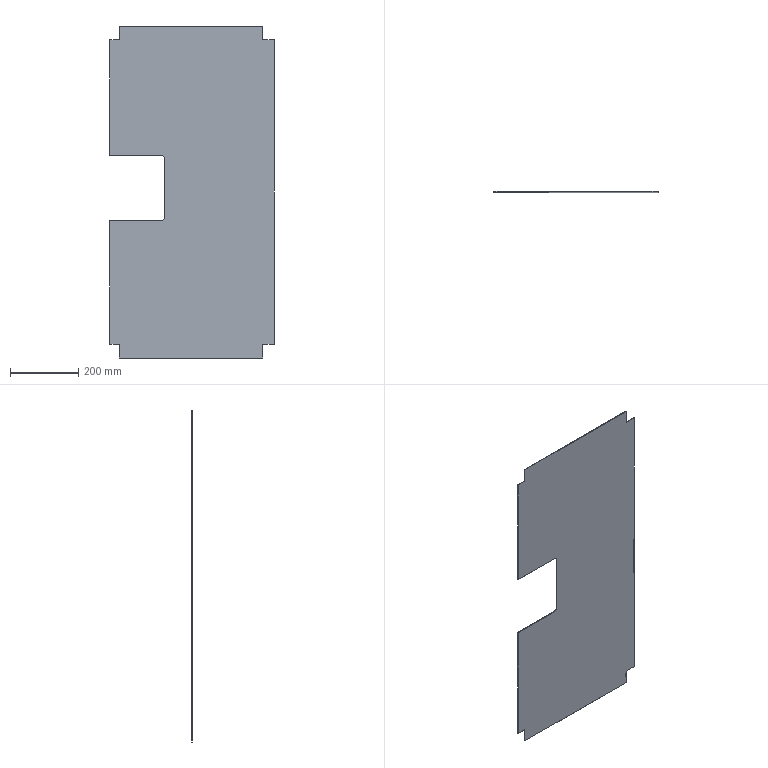Part | SolidWorks | features BaseBody 1 | 1 solid | 20 faces | box 480 x 1.5 x 970 mm | volume 645737 mm3 | plane 18 | cylinder 2 | commonest cylinder face diameters 20 x2
STEP:
#1=CARTESIAN_POINT('',(-254.,-1.5,-83.686));
#2=VERTEX_POINT('',#1);
#3=CARTESIAN_POINT('',(-104.677,-1.5,-83.686));
#4=VERTEX_POINT('',#3);
#5=CARTESIAN_POINT('',(0.,-1.5,-83.686));
#6=DIRECTION('',(1.,0.,0.));
#7=VECTOR('',#6,1000.);
#8=LINE('',#5,#7);
#9=EDGE_CURVE('',#2,#4,#8,.T.);
#10=ORIENTED_EDGE('',*,*,#9,.F.);
#11=CARTESIAN_POINT('',(-254.,-1.5,-445.));
#12=VERTEX_POINT('',#11);
#13=CARTESIAN_POINT('',(-254.,-1.5,0.));
#14=DIRECTION('',(0.,0.,1.));
#15=VECTOR('',#14,1000.);
#16=LINE('',#13,#15);
#17=EDGE_CURVE('',#12,#2,#16,.T.);
#18=ORIENTED_EDGE('',*,*,#17,.F.);
#19=CARTESIAN_POINT('',(-226.,-1.5,-445.));
#20=VERTEX_POINT('',#19);
#21=CARTESIAN_POINT('',(0.,-1.5,-445.));
#22=DIRECTION('',(-1.,0.,0.));
#23=VECTOR('',#22,1000.);
#24=LINE('',#21,#23);
#25=EDGE_CURVE('',#20,#12,#24,.T.);
#26=ORIENTED_EDGE('',*,*,#25,.F.);
#27=CARTESIAN_POINT('',(-226.,-1.5,-485.));
#28=VERTEX_POINT('',#27);
#29=CARTESIAN_POINT('',(-226.,-1.5,0.));
#30=DIRECTION('',(0.,0.,1.));
#31=VECTOR('',#30,1000.);
#32=LINE('',#29,#31);
#33=EDGE_CURVE('',#28,#20,#32,.T.);
#34=ORIENTED_EDGE('',*,*,#33,.F.);
#35=CARTESIAN_POINT('',(193.,-1.5,-485.));
#36=VERTEX_POINT('',#35);
#37=CARTESIAN_POINT('',(0.,-1.5,-485.));
#38=DIRECTION('',(-1.,0.,0.));
#39=VECTOR('',#38,1000.);
#40=LINE('',#37,#39);
#41=EDGE_CURVE('',#36,#28,#40,.T.);
#42=ORIENTED_EDGE('',*,*,#41,.F.);
#43=CARTESIAN_POINT('',(193.,-1.5,-445.));
#44=VERTEX_POINT('',#43);
#45=CARTESIAN_POINT('',(193.,-1.5,0.));
#46=DIRECTION('',(0.,0.,-1.));
#47=VECTOR('',#46,1000.);
#48=LINE('',#45,#47);
#49=EDGE_CURVE('',#44,#36,#48,.T.);
#50=ORIENTED_EDGE('',*,*,#49,.F.);
#51=CARTESIAN_POINT('',(226.,-1.5,-445.));
#52=VERTEX_POINT('',#51);
#53=CARTESIAN_POINT('',(0.,-1.5,-445.));
#54=DIRECTION('',(-1.,0.,0.));
#55=VECTOR('',#54,1000.);
#56=LINE('',#53,#55);
#57=EDGE_CURVE('',#52,#44,#56,.T.);
#58=ORIENTED_EDGE('',*,*,#57,.F.);
#59=CARTESIAN_POINT('',(226.,-1.5,445.));
#60=VERTEX_POINT('',#59);
#61=CARTESIAN_POINT('',(226.,-1.5,0.));
#62=DIRECTION('',(0.,0.,-1.));
#63=VECTOR('',#62,1000.);
#64=LINE('',#61,#63);
#65=EDGE_CURVE('',#60,#52,#64,.T.);
#66=ORIENTED_EDGE('',*,*,#65,.F.);
#67=CARTESIAN_POINT('',(193.,-1.5,445.));
#68=VERTEX_POINT('',#67);
#69=CARTESIAN_POINT('',(0.,-1.5,445.));
#70=DIRECTION('',(1.,0.,0.));
#71=VECTOR('',#70,1000.);
#72=LINE('',#69,#71);
#73=EDGE_CURVE('',#68,#60,#72,.T.);
#74=ORIENTED_EDGE('',*,*,#73,.F.);
#75=CARTESIAN_POINT('',(193.,-1.5,485.));
#76=VERTEX_POINT('',#75);
#77=CARTESIAN_POINT('',(193.,-1.5,0.));
#78=DIRECTION('',(0.,0.,-1.));
#79=VECTOR('',#78,1000.);
#80=LINE('',#77,#79);
#81=EDGE_CURVE('',#76,#68,#80,.T.);
#82=ORIENTED_EDGE('',*,*,#81,.F.);
#83=CARTESIAN_POINT('',(-226.,-1.5,485.));
#84=VERTEX_POINT('',#83);
#85=CARTESIAN_POINT('',(0.,-1.5,485.));
#86=DIRECTION('',(1.,0.,0.));
#87=VECTOR('',#86,1000.);
#88=LINE('',#85,#87);
#89=EDGE_CURVE('',#84,#76,#88,.T.);
#90=ORIENTED_EDGE('',*,*,#89,.F.);
#91=CARTESIAN_POINT('',(-226.,-1.5,445.));
#92=VERTEX_POINT('',#91);
#93=CARTESIAN_POINT('',(-226.,-1.5,0.));
#94=DIRECTION('',(0.,0.,1.));
#95=VECTOR('',#94,1000.);
#96=LINE('',#93,#95);
#97=EDGE_CURVE('',#92,#84,#96,.T.);
#98=ORIENTED_EDGE('',*,*,#97,.F.);
#99=CARTESIAN_POINT('',(-254.,-1.5,445.));
#100=VERTEX_POINT('',#99);
#101=CARTESIAN_POINT('',(0.,-1.5,445.));
#102=DIRECTION('',(1.,0.,0.));
#103=VECTOR('',#102,1000.);
#104=LINE('',#101,#103);
#105=EDGE_CURVE('',#100,#92,#104,.T.);
#106=ORIENTED_EDGE('',*,*,#105,.F.);
#107=CARTESIAN_POINT('',(-254.,-1.5,106.314));
#108=VERTEX_POINT('',#107);
#109=CARTESIAN_POINT('',(-254.,-1.5,0.));
#110=DIRECTION('',(0.,0.,1.));
#111=VECTOR('',#110,1000.);
#112=LINE('',#109,#111);
#113=EDGE_CURVE('',#108,#100,#112,.T.);
#114=ORIENTED_EDGE('',*,*,#113,.F.);
#115=CARTESIAN_POINT('',(-104.677,-1.5,106.314));
#116=VERTEX_POINT('',#115);
#117=CARTESIAN_POINT('',(0.,-1.5,106.314));
#118=DIRECTION('',(-1.,0.,0.));
#119=VECTOR('',#118,1000.);
#120=LINE('',#117,#119);
#121=EDGE_CURVE('',#116,#108,#120,.T.);
#122=ORIENTED_EDGE('',*,*,#121,.F.);
#123=CARTESIAN_POINT('',(-94.677,-1.5,96.314));
#124=VERTEX_POINT('',#123);
#125=CARTESIAN_POINT('',(-104.677,-1.5,96.314));
#126=DIRECTION('',(0.,-1.,0.));
#127=DIRECTION('',(0.,0.,1.));
#128=AXIS2_PLACEMENT_3D('',#125,#126,#127);
#129=CIRCLE('',#128,10.);
#130=EDGE_CURVE('',#124,#116,#129,.T.);
#131=ORIENTED_EDGE('',*,*,#130,.F.);
#132=CARTESIAN_POINT('',(-94.677,-1.5,-73.686));
#133=VERTEX_POINT('',#132);
#134=CARTESIAN_POINT('',(-94.677,-1.5,0.));
#135=DIRECTION('',(0.,0.,1.));
#136=VECTOR('',#135,1000.);
#137=LINE('',#134,#136);
#138=EDGE_CURVE('',#133,#124,#137,.T.);
#139=ORIENTED_EDGE('',*,*,#138,.F.);
#140=CARTESIAN_POINT('',(-104.677,-1.5,-73.686));
#141=DIRECTION('',(0.,-1.,0.));
#142=DIRECTION('',(0.,0.,1.));
#143=AXIS2_PLACEMENT_3D('',#140,#141,#142);
#144=CIRCLE('',#143,10.);
#145=EDGE_CURVE('',#4,#133,#144,.T.);
#146=ORIENTED_EDGE('',*,*,#145,.F.);
#147=EDGE_LOOP('',(#10,#18,#26,#34,#42,#50,#58,#66,#74,#82,#90,#98,#106,#114,#122,#131,#139,#146));
#148=FACE_OUTER_BOUND('',#147,.T.);
#149=CARTESIAN_POINT('',(0.,-1.5,0.));
#150=DIRECTION('',(0.,1.,0.));
#151=DIRECTION('',(0.,0.,1.));
#152=AXIS2_PLACEMENT_3D('',#149,#150,#151);
#153=PLANE('',#152);
#154=ADVANCED_FACE('',(#148),#153,.F.);
#155=CARTESIAN_POINT('',(-104.677,0.,-83.686));
#156=VERTEX_POINT('',#155);
#157=CARTESIAN_POINT('',(-94.677,0.,-73.686));
#158=VERTEX_POINT('',#157);
#159=CARTESIAN_POINT('',(-104.677,0.,-73.686));
#160=DIRECTION('',(0.,-1.,0.));
#161=DIRECTION('',(0.,0.,1.));
#162=AXIS2_PLACEMENT_3D('',#159,#160,#161);
#163=CIRCLE('',#162,10.);
#164=EDGE_CURVE('',#156,#158,#163,.T.);
#165=ORIENTED_EDGE('',*,*,#164,.F.);
#166=CARTESIAN_POINT('',(-104.677,-10.,-83.686));
#167=DIRECTION('',(0.,1.,0.));
#168=VECTOR('',#167,1000.);
#169=LINE('',#166,#168);
#170=EDGE_CURVE('',#4,#156,#169,.T.);
#171=ORIENTED_EDGE('',*,*,#170,.F.);
#172=ORIENTED_EDGE('',*,*,#145,.T.);
#173=CARTESIAN_POINT('',(-94.677,-10.,-73.686));
#174=DIRECTION('',(0.,-1.,0.));
#175=VECTOR('',#174,1000.);
#176=LINE('',#173,#175);
#177=EDGE_CURVE('',#158,#133,#176,.T.);
#178=ORIENTED_EDGE('',*,*,#177,.F.);
#179=EDGE_LOOP('',(#165,#171,#172,#178));
#180=FACE_OUTER_BOUND('',#179,.T.);
#181=CARTESIAN_POINT('',(-104.677,-10.,-73.686));
#182=DIRECTION('',(0.,1.,0.));
#183=DIRECTION('',(0.,0.,1.));
#184=AXIS2_PLACEMENT_3D('',#181,#182,#183);
#185=CYLINDRICAL_SURFACE('',#184,10.);
#186=ADVANCED_FACE('',(#180),#185,.F.);
#187=ORIENTED_EDGE('',*,*,#9,.T.);
#188=ORIENTED_EDGE('',*,*,#170,.T.);
#189=CARTESIAN_POINT('',(-254.,0.,-83.686));
#190=VERTEX_POINT('',#189);
#191=CARTESIAN_POINT('',(-104.677,0.,-83.686));
#192=DIRECTION('',(1.,0.,0.));
#193=VECTOR('',#192,1000.);
#194=LINE('',#191,#193);
#195=EDGE_CURVE('',#190,#156,#194,.T.);
#196=ORIENTED_EDGE('',*,*,#195,.F.);
#197=CARTESIAN_POINT('',(-254.,-10.,-83.686));
#198=DIRECTION('',(0.,1.,0.));
#199=VECTOR('',#198,1000.);
#200=LINE('',#197,#199);
#201=EDGE_CURVE('',#2,#190,#200,.T.);
#202=ORIENTED_EDGE('',*,*,#201,.F.);
#203=EDGE_LOOP('',(#187,#188,#196,#202));
#204=FACE_OUTER_BOUND('',#203,.T.);
#205=CARTESIAN_POINT('',(-104.677,-10.,-83.686));
#206=DIRECTION('',(0.,0.,-1.));
#207=DIRECTION('',(-1.,0.,0.));
#208=AXIS2_PLACEMENT_3D('',#205,#206,#207);
#209=PLANE('',#208);
#210=ADVANCED_FACE('',(#204),#209,.F.);
#211=CARTESIAN_POINT('',(-254.,0.,-445.));
#212=VERTEX_POINT('',#211);
#213=CARTESIAN_POINT('',(-254.,-1.5,-445.));
#214=DIRECTION('',(0.,-1.,0.));
#215=VECTOR('',#214,1000.);
#216=LINE('',#213,#215);
#217=EDGE_CURVE('',#212,#12,#216,.T.);
#218=ORIENTED_EDGE('',*,*,#217,.T.);
#219=ORIENTED_EDGE('',*,*,#17,.T.);
#220=ORIENTED_EDGE('',*,*,#201,.T.);
#221=CARTESIAN_POINT('',(-254.,0.,445.));
#222=DIRECTION('',(0.,0.,-1.));
#223=VECTOR('',#222,1000.);
#224=LINE('',#221,#223);
#225=EDGE_CURVE('',#190,#212,#224,.T.);
#226=ORIENTED_EDGE('',*,*,#225,.T.);
#227=EDGE_LOOP('',(#218,#219,#220,#226));
#228=FACE_OUTER_BOUND('',#227,.T.);
#229=CARTESIAN_POINT('',(-254.,-1.5,445.));
#230=DIRECTION('',(-1.,0.,0.));
#231=DIRECTION('',(0.,0.,1.));
#232=AXIS2_PLACEMENT_3D('',#229,#230,#231);
#233=PLANE('',#232);
#234=ADVANCED_FACE('',(#228),#233,.T.);
#235=ORIENTED_EDGE('',*,*,#25,.T.);
#236=ORIENTED_EDGE('',*,*,#217,.F.);
#237=CARTESIAN_POINT('',(-226.,0.,-445.));
#238=VERTEX_POINT('',#237);
#239=CARTESIAN_POINT('',(-254.,0.,-445.));
#240=DIRECTION('',(1.,0.,0.));
#241=VECTOR('',#240,1000.);
#242=LINE('',#239,#241);
#243=EDGE_CURVE('',#212,#238,#242,.T.);
#244=ORIENTED_EDGE('',*,*,#243,.T.);
#245=CARTESIAN_POINT('',(-226.,-1.5,-445.));
#246=DIRECTION('',(0.,-1.,0.));
#247=VECTOR('',#246,1000.);
#248=LINE('',#245,#247);
#249=EDGE_CURVE('',#238,#20,#248,.T.);
#250=ORIENTED_EDGE('',*,*,#249,.T.);
#251=EDGE_LOOP('',(#235,#236,#244,#250));
#252=FACE_OUTER_BOUND('',#251,.T.);
#253=CARTESIAN_POINT('',(-254.,-1.5,-445.));
#254=DIRECTION('',(0.,0.,-1.));
#255=DIRECTION('',(-1.,0.,0.));
#256=AXIS2_PLACEMENT_3D('',#253,#254,#255);
#257=PLANE('',#256);
#258=ADVANCED_FACE('',(#252),#257,.T.);
#259=ORIENTED_EDGE('',*,*,#33,.T.);
#260=ORIENTED_EDGE('',*,*,#249,.F.);
#261=CARTESIAN_POINT('',(-226.,0.,-485.));
#262=VERTEX_POINT('',#261);
#263=CARTESIAN_POINT('',(-226.,0.,-445.));
#264=DIRECTION('',(0.,0.,-1.));
#265=VECTOR('',#264,1000.);
#266=LINE('',#263,#265);
#267=EDGE_CURVE('',#238,#262,#266,.T.);
#268=ORIENTED_EDGE('',*,*,#267,.T.);
#269=CARTESIAN_POINT('',(-226.,-1.5,-485.));
#270=DIRECTION('',(0.,-1.,0.));
#271=VECTOR('',#270,1000.);
#272=LINE('',#269,#271);
#273=EDGE_CURVE('',#262,#28,#272,.T.);
#274=ORIENTED_EDGE('',*,*,#273,.T.);
#275=EDGE_LOOP('',(#259,#260,#268,#274));
#276=FACE_OUTER_BOUND('',#275,.T.);
#277=CARTESIAN_POINT('',(-226.,-1.5,-445.));
#278=DIRECTION('',(-1.,0.,0.));
#279=DIRECTION('',(0.,0.,1.));
#280=AXIS2_PLACEMENT_3D('',#277,#278,#279);
#281=PLANE('',#280);
#282=ADVANCED_FACE('',(#276),#281,.T.);
#283=ORIENTED_EDGE('',*,*,#41,.T.);
#284=ORIENTED_EDGE('',*,*,#273,.F.);
#285=CARTESIAN_POINT('',(193.,0.,-485.));
#286=VERTEX_POINT('',#285);
#287=CARTESIAN_POINT('',(-226.,0.,-485.));
#288=DIRECTION('',(1.,0.,0.));
#289=VECTOR('',#288,1000.);
#290=LINE('',#287,#289);
#291=EDGE_CURVE('',#262,#286,#290,.T.);
#292=ORIENTED_EDGE('',*,*,#291,.T.);
#293=CARTESIAN_POINT('',(193.,-1.5,-485.));
#294=DIRECTION('',(0.,-1.,0.));
#295=VECTOR('',#294,1000.);
#296=LINE('',#293,#295);
#297=EDGE_CURVE('',#286,#36,#296,.T.);
#298=ORIENTED_EDGE('',*,*,#297,.T.);
#299=EDGE_LOOP('',(#283,#284,#292,#298));
#300=FACE_OUTER_BOUND('',#299,.T.);
#301=CARTESIAN_POINT('',(-226.,-1.5,-485.));
#302=DIRECTION('',(0.,0.,-1.));
#303=DIRECTION('',(-1.,0.,0.));
#304=AXIS2_PLACEMENT_3D('',#301,#302,#303);
#305=PLANE('',#304);
#306=ADVANCED_FACE('',(#300),#305,.T.);
#307=ORIENTED_EDGE('',*,*,#49,.T.);
#308=ORIENTED_EDGE('',*,*,#297,.F.);
#309=CARTESIAN_POINT('',(193.,0.,-445.));
#310=VERTEX_POINT('',#309);
#311=CARTESIAN_POINT('',(193.,0.,-485.));
#312=DIRECTION('',(0.,0.,1.));
#313=VECTOR('',#312,1000.);
#314=LINE('',#311,#313);
#315=EDGE_CURVE('',#286,#310,#314,.T.);
#316=ORIENTED_EDGE('',*,*,#315,.T.);
#317=CARTESIAN_POINT('',(193.,-1.5,-445.));
#318=DIRECTION('',(0.,-1.,0.));
#319=VECTOR('',#318,1000.);
#320=LINE('',#317,#319);
#321=EDGE_CURVE('',#310,#44,#320,.T.);
#322=ORIENTED_EDGE('',*,*,#321,.T.);
#323=EDGE_LOOP('',(#307,#308,#316,#322));
#324=FACE_OUTER_BOUND('',#323,.T.);
#325=CARTESIAN_POINT('',(193.,-1.5,-485.));
#326=DIRECTION('',(1.,0.,0.));
#327=DIRECTION('',(0.,0.,-1.));
#328=AXIS2_PLACEMENT_3D('',#325,#326,#327);
#329=PLANE('',#328);
#330=ADVANCED_FACE('',(#324),#329,.T.);
#331=ORIENTED_EDGE('',*,*,#57,.T.);
#332=ORIENTED_EDGE('',*,*,#321,.F.);
#333=CARTESIAN_POINT('',(226.,0.,-445.));
#334=VERTEX_POINT('',#333);
#335=CARTESIAN_POINT('',(226.,0.,-445.));
#336=DIRECTION('',(1.,0.,0.));
#337=VECTOR('',#336,1000.);
#338=LINE('',#335,#337);
#339=EDGE_CURVE('',#310,#334,#338,.T.);
#340=ORIENTED_EDGE('',*,*,#339,.T.);
#341=CARTESIAN_POINT('',(226.,-1.5,-445.));
#342=DIRECTION('',(0.,-1.,0.));
#343=VECTOR('',#342,1000.);
#344=LINE('',#341,#343);
#345=EDGE_CURVE('',#334,#52,#344,.T.);
#346=ORIENTED_EDGE('',*,*,#345,.T.);
#347=EDGE_LOOP('',(#331,#332,#340,#346));
#348=FACE_OUTER_BOUND('',#347,.T.);
#349=CARTESIAN_POINT('',(226.,-1.5,-445.));
#350=DIRECTION('',(0.,0.,-1.));
#351=DIRECTION('',(-1.,0.,0.));
#352=AXIS2_PLACEMENT_3D('',#349,#350,#351);
#353=PLANE('',#352);
#354=ADVANCED_FACE('',(#348),#353,.T.);
#355=ORIENTED_EDGE('',*,*,#65,.T.);
#356=ORIENTED_EDGE('',*,*,#345,.F.);
#357=CARTESIAN_POINT('',(226.,0.,445.));
#358=VERTEX_POINT('',#357);
#359=CARTESIAN_POINT('',(226.,0.,445.));
#360=DIRECTION('',(0.,0.,1.));
#361=VECTOR('',#360,1000.);
#362=LINE('',#359,#361);
#363=EDGE_CURVE('',#334,#358,#362,.T.);
#364=ORIENTED_EDGE('',*,*,#363,.T.);
#365=CARTESIAN_POINT('',(226.,-1.5,445.));
#366=DIRECTION('',(0.,-1.,0.));
#367=VECTOR('',#366,1000.);
#368=LINE('',#365,#367);
#369=EDGE_CURVE('',#358,#60,#368,.T.);
#370=ORIENTED_EDGE('',*,*,#369,.T.);
#371=EDGE_LOOP('',(#355,#356,#364,#370));
#372=FACE_OUTER_BOUND('',#371,.T.);
#373=CARTESIAN_POINT('',(226.,-1.5,445.));
#374=DIRECTION('',(1.,0.,0.));
#375=DIRECTION('',(0.,0.,-1.));
#376=AXIS2_PLACEMENT_3D('',#373,#374,#375);
#377=PLANE('',#376);
#378=ADVANCED_FACE('',(#372),#377,.T.);
#379=ORIENTED_EDGE('',*,*,#73,.T.);
#380=ORIENTED_EDGE('',*,*,#369,.F.);
#381=CARTESIAN_POINT('',(193.,0.,445.));
#382=VERTEX_POINT('',#381);
#383=CARTESIAN_POINT('',(226.,0.,445.));
#384=DIRECTION('',(-1.,0.,0.));
#385=VECTOR('',#384,1000.);
#386=LINE('',#383,#385);
#387=EDGE_CURVE('',#358,#382,#386,.T.);
#388=ORIENTED_EDGE('',*,*,#387,.T.);
#389=CARTESIAN_POINT('',(193.,-1.5,445.));
#390=DIRECTION('',(0.,-1.,0.));
#391=VECTOR('',#390,1000.);
#392=LINE('',#389,#391);
#393=EDGE_CURVE('',#382,#68,#392,.T.);
#394=ORIENTED_EDGE('',*,*,#393,.T.);
#395=EDGE_LOOP('',(#379,#380,#388,#394));
#396=FACE_OUTER_BOUND('',#395,.T.);
#397=CARTESIAN_POINT('',(226.,-1.5,445.));
#398=DIRECTION('',(0.,0.,1.));
#399=DIRECTION('',(1.,0.,0.));
#400=AXIS2_PLACEMENT_3D('',#397,#398,#399);
#401=PLANE('',#400);
#402=ADVANCED_FACE('',(#396),#401,.T.);
#403=ORIENTED_EDGE('',*,*,#81,.T.);
#404=ORIENTED_EDGE('',*,*,#393,.F.);
#405=CARTESIAN_POINT('',(193.,0.,485.));
#406=VERTEX_POINT('',#405);
#407=CARTESIAN_POINT('',(193.,0.,485.));
#408=DIRECTION('',(0.,0.,1.));
#409=VECTOR('',#408,1000.);
#410=LINE('',#407,#409);
#411=EDGE_CURVE('',#382,#406,#410,.T.);
#412=ORIENTED_EDGE('',*,*,#411,.T.);
#413=CARTESIAN_POINT('',(193.,-1.5,485.));
#414=DIRECTION('',(0.,-1.,0.));
#415=VECTOR('',#414,1000.);
#416=LINE('',#413,#415);
#417=EDGE_CURVE('',#406,#76,#416,.T.);
#418=ORIENTED_EDGE('',*,*,#417,.T.);
#419=EDGE_LOOP('',(#403,#404,#412,#418));
#420=FACE_OUTER_BOUND('',#419,.T.);
#421=CARTESIAN_POINT('',(193.,-1.5,485.));
#422=DIRECTION('',(1.,0.,0.));
#423=DIRECTION('',(0.,0.,-1.));
#424=AXIS2_PLACEMENT_3D('',#421,#422,#423);
#425=PLANE('',#424);
#426=ADVANCED_FACE('',(#420),#425,.T.);
#427=ORIENTED_EDGE('',*,*,#89,.T.);
#428=ORIENTED_EDGE('',*,*,#417,.F.);
#429=CARTESIAN_POINT('',(-226.,0.,485.));
#430=VERTEX_POINT('',#429);
#431=CARTESIAN_POINT('',(-226.,0.,485.));
#432=DIRECTION('',(-1.,0.,0.));
#433=VECTOR('',#432,1000.);
#434=LINE('',#431,#433);
#435=EDGE_CURVE('',#406,#430,#434,.T.);
#436=ORIENTED_EDGE('',*,*,#435,.T.);
#437=CARTESIAN_POINT('',(-226.,-1.5,485.));
#438=DIRECTION('',(0.,-1.,0.));
#439=VECTOR('',#438,1000.);
#440=LINE('',#437,#439);
#441=EDGE_CURVE('',#430,#84,#440,.T.);
#442=ORIENTED_EDGE('',*,*,#441,.T.);
#443=EDGE_LOOP('',(#427,#428,#436,#442));
#444=FACE_OUTER_BOUND('',#443,.T.);
#445=CARTESIAN_POINT('',(-226.,-1.5,485.));
#446=DIRECTION('',(0.,0.,1.));
#447=DIRECTION('',(1.,0.,0.));
#448=AXIS2_PLACEMENT_3D('',#445,#446,#447);
#449=PLANE('',#448);
#450=ADVANCED_FACE('',(#444),#449,.T.);
#451=ORIENTED_EDGE('',*,*,#97,.T.);
#452=ORIENTED_EDGE('',*,*,#441,.F.);
#453=CARTESIAN_POINT('',(-226.,0.,445.));
#454=VERTEX_POINT('',#453);
#455=CARTESIAN_POINT('',(-226.,0.,485.));
#456=DIRECTION('',(0.,0.,-1.));
#457=VECTOR('',#456,1000.);
#458=LINE('',#455,#457);
#459=EDGE_CURVE('',#430,#454,#458,.T.);
#460=ORIENTED_EDGE('',*,*,#459,.T.);
#461=CARTESIAN_POINT('',(-226.,-1.5,445.));
#462=DIRECTION('',(0.,-1.,0.));
#463=VECTOR('',#462,1000.);
#464=LINE('',#461,#463);
#465=EDGE_CURVE('',#454,#92,#464,.T.);
#466=ORIENTED_EDGE('',*,*,#465,.T.);
#467=EDGE_LOOP('',(#451,#452,#460,#466));
#468=FACE_OUTER_BOUND('',#467,.T.);
#469=CARTESIAN_POINT('',(-226.,-1.5,485.));
#470=DIRECTION('',(-1.,0.,0.));
#471=DIRECTION('',(0.,0.,1.));
#472=AXIS2_PLACEMENT_3D('',#469,#470,#471);
#473=PLANE('',#472);
#474=ADVANCED_FACE('',(#468),#473,.T.);
#475=ORIENTED_EDGE('',*,*,#105,.T.);
#476=ORIENTED_EDGE('',*,*,#465,.F.);
#477=CARTESIAN_POINT('',(-254.,0.,445.));
#478=VERTEX_POINT('',#477);
#479=CARTESIAN_POINT('',(-226.,0.,445.));
#480=DIRECTION('',(-1.,0.,0.));
#481=VECTOR('',#480,1000.);
#482=LINE('',#479,#481);
#483=EDGE_CURVE('',#454,#478,#482,.T.);
#484=ORIENTED_EDGE('',*,*,#483,.T.);
#485=CARTESIAN_POINT('',(-254.,-1.5,445.));
#486=DIRECTION('',(0.,-1.,0.));
#487=VECTOR('',#486,1000.);
#488=LINE('',#485,#487);
#489=EDGE_CURVE('',#478,#100,#488,.T.);
#490=ORIENTED_EDGE('',*,*,#489,.T.);
#491=EDGE_LOOP('',(#475,#476,#484,#490));
#492=FACE_OUTER_BOUND('',#491,.T.);
#493=CARTESIAN_POINT('',(-226.,-1.5,445.));
#494=DIRECTION('',(0.,0.,1.));
#495=DIRECTION('',(1.,0.,0.));
#496=AXIS2_PLACEMENT_3D('',#493,#494,#495);
#497=PLANE('',#496);
#498=ADVANCED_FACE('',(#492),#497,.T.);
#499=ORIENTED_EDGE('',*,*,#489,.F.);
#500=CARTESIAN_POINT('',(-254.,0.,106.314));
#501=VERTEX_POINT('',#500);
#502=CARTESIAN_POINT('',(-254.,0.,445.));
#503=DIRECTION('',(0.,0.,-1.));
#504=VECTOR('',#503,1000.);
#505=LINE('',#502,#504);
#506=EDGE_CURVE('',#478,#501,#505,.T.);
#507=ORIENTED_EDGE('',*,*,#506,.T.);
#508=CARTESIAN_POINT('',(-254.,-1.5,106.314));
#509=DIRECTION('',(0.,-1.,0.));
#510=VECTOR('',#509,1000.);
#511=LINE('',#508,#510);
#512=EDGE_CURVE('',#501,#108,#511,.T.);
#513=ORIENTED_EDGE('',*,*,#512,.T.);
#514=ORIENTED_EDGE('',*,*,#113,.T.);
#515=EDGE_LOOP('',(#499,#507,#513,#514));
#516=FACE_OUTER_BOUND('',#515,.T.);
#517=CARTESIAN_POINT('',(-254.,-1.5,445.));
#518=DIRECTION('',(-1.,0.,0.));
#519=DIRECTION('',(0.,0.,1.));
#520=AXIS2_PLACEMENT_3D('',#517,#518,#519);
#521=PLANE('',#520);
#522=ADVANCED_FACE('',(#516),#521,.T.);
#523=CARTESIAN_POINT('',(-104.677,0.,106.314));
#524=VERTEX_POINT('',#523);
#525=CARTESIAN_POINT('',(-394.677,0.,106.314));
#526=DIRECTION('',(-1.,0.,0.));
#527=VECTOR('',#526,1000.);
#528=LINE('',#525,#527);
#529=EDGE_CURVE('',#524,#501,#528,.T.);
#530=ORIENTED_EDGE('',*,*,#529,.F.);
#531=CARTESIAN_POINT('',(-104.677,-10.,106.314));
#532=DIRECTION('',(0.,1.,0.));
#533=VECTOR('',#532,1000.);
#534=LINE('',#531,#533);
#535=EDGE_CURVE('',#116,#524,#534,.T.);
#536=ORIENTED_EDGE('',*,*,#535,.F.);
#537=ORIENTED_EDGE('',*,*,#121,.T.);
#538=ORIENTED_EDGE('',*,*,#512,.F.);
#539=EDGE_LOOP('',(#530,#536,#537,#538));
#540=FACE_OUTER_BOUND('',#539,.T.);
#541=CARTESIAN_POINT('',(-394.677,-10.,106.314));
#542=DIRECTION('',(0.,0.,1.));
#543=DIRECTION('',(1.,0.,0.));
#544=AXIS2_PLACEMENT_3D('',#541,#542,#543);
#545=PLANE('',#544);
#546=ADVANCED_FACE('',(#540),#545,.F.);
#547=CARTESIAN_POINT('',(-94.677,0.,96.314));
#548=VERTEX_POINT('',#547);
#549=CARTESIAN_POINT('',(-104.677,0.,96.314));
#550=DIRECTION('',(0.,-1.,0.));
#551=DIRECTION('',(0.,0.,1.));
#552=AXIS2_PLACEMENT_3D('',#549,#550,#551);
#553=CIRCLE('',#552,10.);
#554=EDGE_CURVE('',#548,#524,#553,.T.);
#555=ORIENTED_EDGE('',*,*,#554,.F.);
#556=CARTESIAN_POINT('',(-94.677,-10.,96.314));
#557=DIRECTION('',(0.,1.,0.));
#558=VECTOR('',#557,1000.);
#559=LINE('',#556,#558);
#560=EDGE_CURVE('',#124,#548,#559,.T.);
#561=ORIENTED_EDGE('',*,*,#560,.F.);
#562=ORIENTED_EDGE('',*,*,#130,.T.);
#563=ORIENTED_EDGE('',*,*,#535,.T.);
#564=EDGE_LOOP('',(#555,#561,#562,#563));
#565=FACE_OUTER_BOUND('',#564,.T.);
#566=CARTESIAN_POINT('',(-104.677,-10.,96.314));
#567=DIRECTION('',(0.,1.,0.));
#568=DIRECTION('',(0.,0.,1.));
#569=AXIS2_PLACEMENT_3D('',#566,#567,#568);
#570=CYLINDRICAL_SURFACE('',#569,10.);
#571=ADVANCED_FACE('',(#565),#570,.F.);
#572=CARTESIAN_POINT('',(-94.677,0.,96.314));
#573=DIRECTION('',(0.,0.,1.));
#574=VECTOR('',#573,1000.);
#575=LINE('',#572,#574);
#576=EDGE_CURVE('',#158,#548,#575,.T.);
#577=ORIENTED_EDGE('',*,*,#576,.F.);
#578=ORIENTED_EDGE('',*,*,#177,.T.);
#579=ORIENTED_EDGE('',*,*,#138,.T.);
#580=ORIENTED_EDGE('',*,*,#560,.T.);
#581=EDGE_LOOP('',(#577,#578,#579,#580));
#582=FACE_OUTER_BOUND('',#581,.T.);
#583=CARTESIAN_POINT('',(-94.677,-10.,96.314));
#584=DIRECTION('',(1.,0.,0.));
#585=DIRECTION('',(0.,0.,-1.));
#586=AXIS2_PLACEMENT_3D('',#583,#584,#585);
#587=PLANE('',#586);
#588=ADVANCED_FACE('',(#582),#587,.F.);
#589=ORIENTED_EDGE('',*,*,#243,.F.);
#590=ORIENTED_EDGE('',*,*,#225,.F.);
#591=ORIENTED_EDGE('',*,*,#195,.T.);
#592=ORIENTED_EDGE('',*,*,#164,.T.);
#593=ORIENTED_EDGE('',*,*,#576,.T.);
#594=ORIENTED_EDGE('',*,*,#554,.T.);
#595=ORIENTED_EDGE('',*,*,#529,.T.);
#596=ORIENTED_EDGE('',*,*,#506,.F.);
#597=ORIENTED_EDGE('',*,*,#483,.F.);
#598=ORIENTED_EDGE('',*,*,#459,.F.);
#599=ORIENTED_EDGE('',*,*,#435,.F.);
#600=ORIENTED_EDGE('',*,*,#411,.F.);
#601=ORIENTED_EDGE('',*,*,#387,.F.);
#602=ORIENTED_EDGE('',*,*,#363,.F.);
#603=ORIENTED_EDGE('',*,*,#339,.F.);
#604=ORIENTED_EDGE('',*,*,#315,.F.);
#605=ORIENTED_EDGE('',*,*,#291,.F.);
#606=ORIENTED_EDGE('',*,*,#267,.F.);
#607=EDGE_LOOP('',(#589,#590,#591,#592,#593,#594,#595,#596,#597,#598,#599,#600,#601,#602,#603,#604,#605,#606));
#608=FACE_OUTER_BOUND('',#607,.T.);
#609=CARTESIAN_POINT('',(0.,0.,0.));
#610=DIRECTION('',(0.,1.,0.));
#611=DIRECTION('',(0.,0.,1.));
#612=AXIS2_PLACEMENT_3D('',#609,#610,#611);
#613=PLANE('',#612);
#614=ADVANCED_FACE('',(#608),#613,.T.);
#615=CLOSED_SHELL('',(#154,#186,#210,#234,#258,#282,#306,#330,#354,#378,#402,#426,#450,#474,#498,#522,#546,#571,#588,#614));
#616=MANIFOLD_SOLID_BREP('',#615);
#617=CARTESIAN_POINT('',(0.,0.,0.));
#618=DIRECTION('',(0.,0.,1.));
#619=DIRECTION('',(1.,0.,0.));
#620=AXIS2_PLACEMENT_3D('',#617,#618,#619);
#621=(LENGTH_UNIT()NAMED_UNIT(*)SI_UNIT(.MILLI.,.METRE.));
#622=UNCERTAINTY_MEASURE_WITH_UNIT(LENGTH_MEASURE(0.00001),#621,'','');
#623=(NAMED_UNIT(*)PLANE_ANGLE_UNIT()SI_UNIT($,.RADIAN.));
#624=(NAMED_UNIT(*)SI_UNIT($,.STERADIAN.)SOLID_ANGLE_UNIT());
#625=(GEOMETRIC_REPRESENTATION_CONTEXT(3)GLOBAL_UNCERTAINTY_ASSIGNED_CONTEXT((#622))GLOBAL_UNIT_ASSIGNED_CONTEXT((#621,#623,#624))REPRESENTATION_CONTEXT('',''));
#626=ADVANCED_BREP_SHAPE_REPRESENTATION('',(#616,#620),#625);